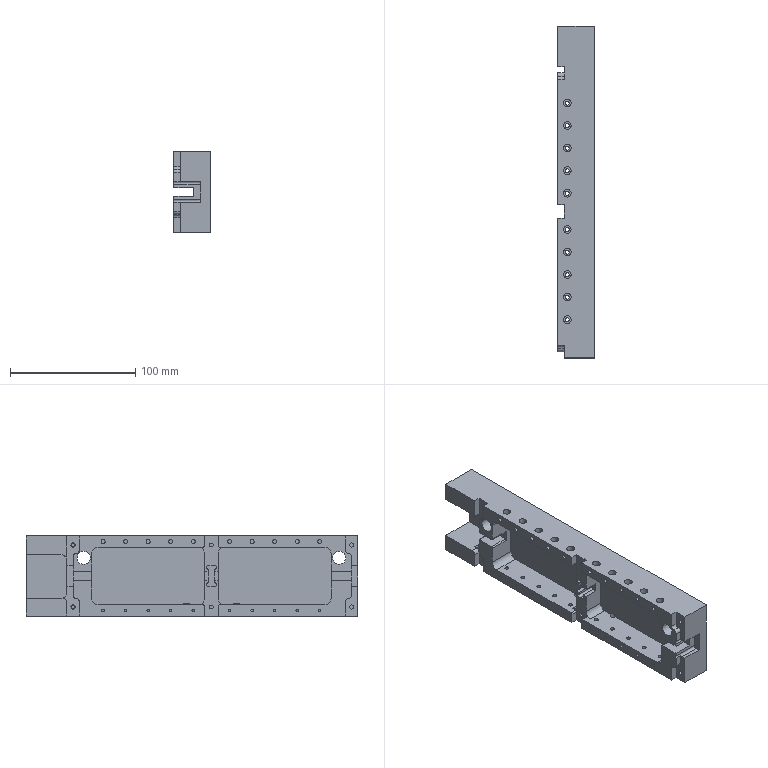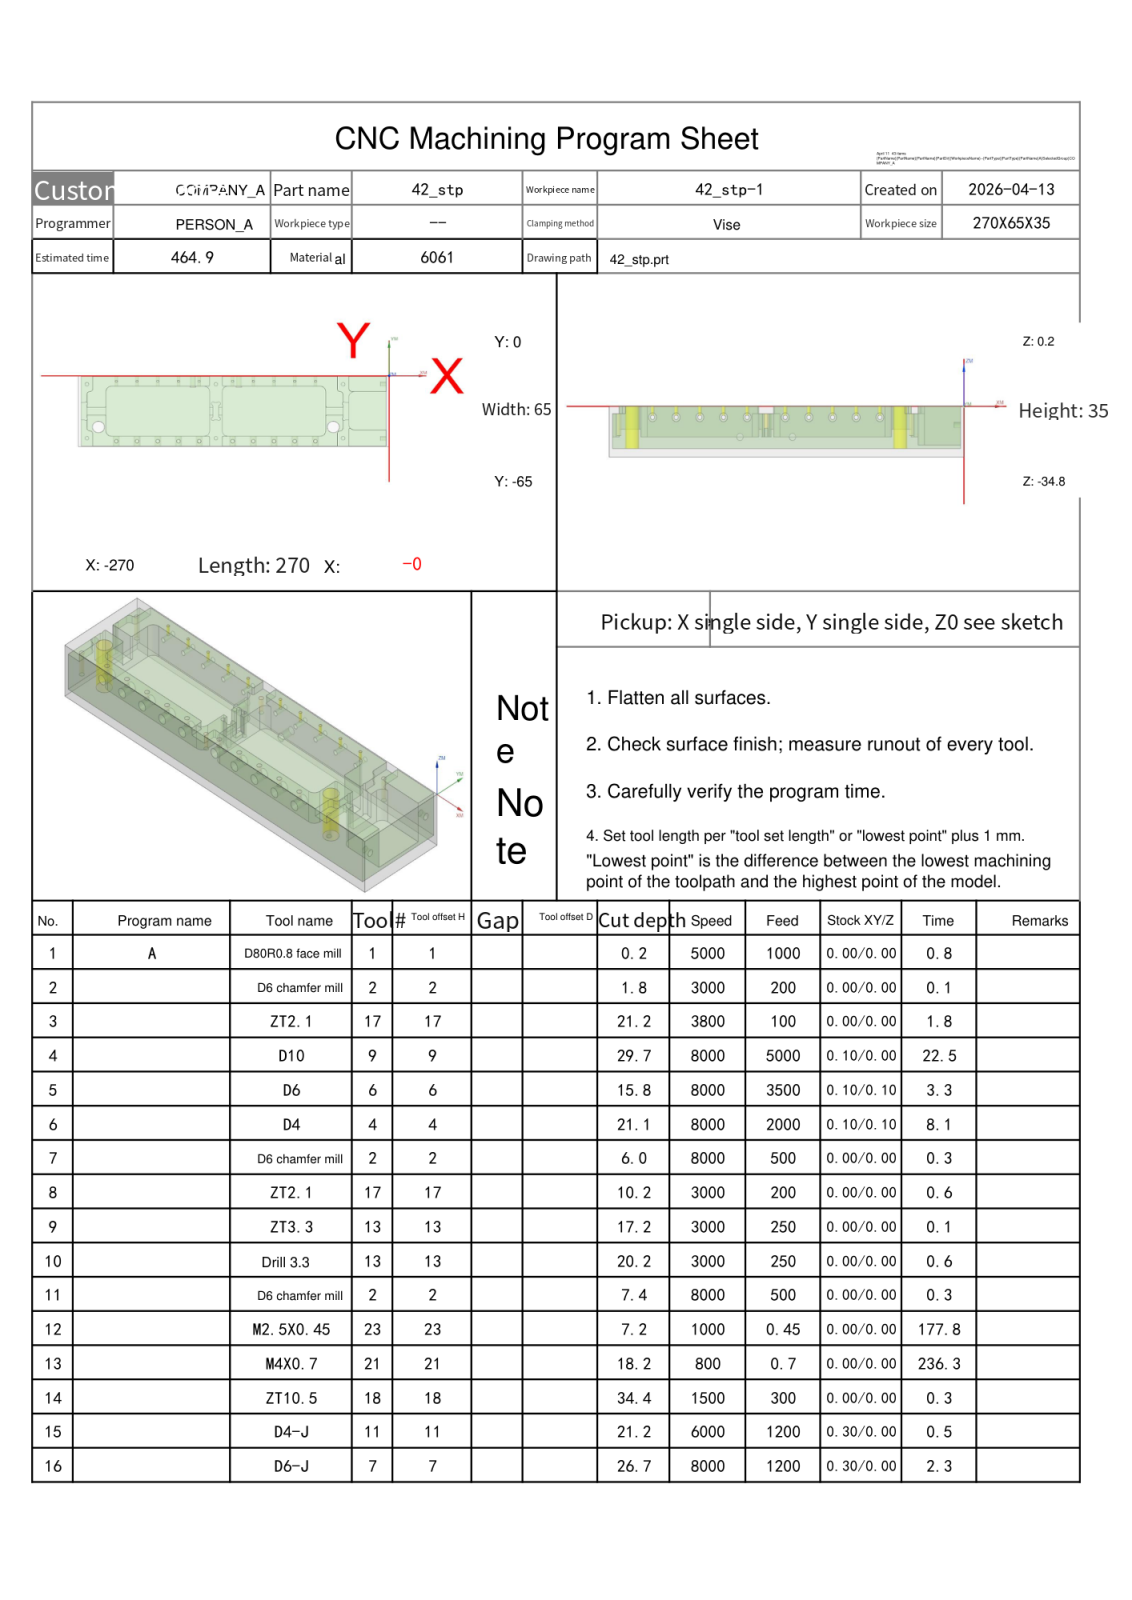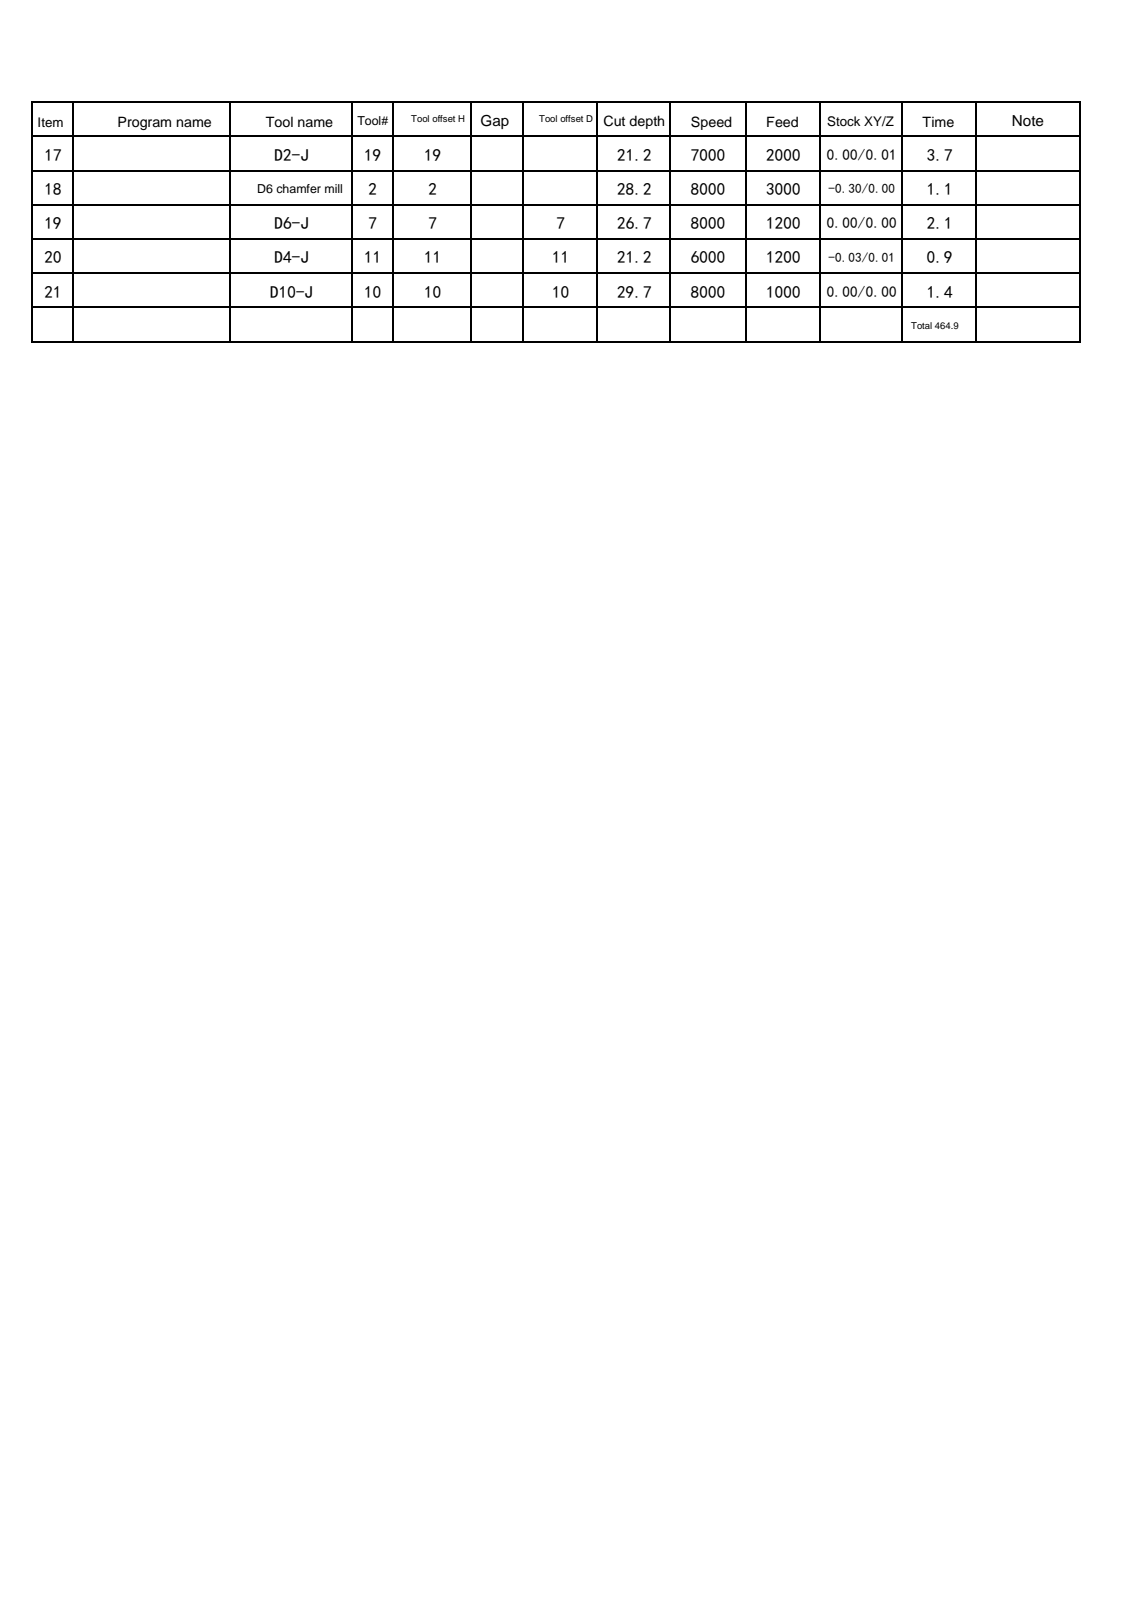NC program | NX | posted by the shop | part box 29 x 265 x 64 mm
Lines 4066 to 6964 of 41846, first 1762 of 2899 lines:
N5 T06 M06
(D6  D=6. R=0. H=06 ce=0.10 di=0.10)
G00 G90 G54 X-162. Y-32.5 M03 S8000
G43 H06 Z10.2
M08
Z1.01
G01 Z-.49 F3000.
X-158.94
Y-14.5
G03 X-160.204 Y-12.6 I-2.06 J0.0
G01 X-157.05
G03 X-153.079 Y-9.522 I0.0 J4.1
G02 X-152.578 Y-9.134 I.501 J-.129
G01 X-152.48 Y-9.143
X-152.325 Y-9.173
X-152.212 Y-9.184
G03 X-151.723 Y-8.931 I0.0 J.6
G02 X-150.5 Y-8.3 I1.223 J-.869
X-149. Y-9.8 I0.0 J-1.5
G01 Y-12.8
G02 X-150.5 Y-14.3 I-1.5 J0.0
X-152. Y-12.8 I0.0 J1.5
G01 Y-10.87
G03 X-152.507 Y-10.278 I-.6 J0.0
G01 X-152.591 Y-10.264
G02 X-153.098 Y-9.672 I.093 J.593
G01 X-153.079 Y-9.522
G03 X-152.95 Y-8.5 I-3.971 J1.022
G01 Y2.44
X-148.05
Y-8.5
G03 X-143.95 Y-12.6 I4.1 J0.0
G01 X-140.796
G03 X-142.06 Y-14.5 I.796 J-1.9
G01 Y-50.5
G03 X-140.796 Y-52.4 I2.06 J0.0
G01 X-143.95
G03 X-147.921 Y-55.478 I0.0 J-4.1
G02 X-148.422 Y-55.866 I-.501 J.129
G01 X-148.52 Y-55.857
X-148.675 Y-55.827
X-148.788 Y-55.816
G03 X-149.277 Y-56.069 I0.0 J-.6
G02 X-150.5 Y-56.7 I-1.223 J.869
X-152. Y-55.2 I0.0 J1.5
G01 Y-52.2
G02 X-150.5 Y-50.7 I1.5 J0.0
X-149. Y-52.2 I0.0 J-1.5
G01 Y-54.13
G03 X-148.493 Y-54.722 I.6 J0.0
G01 X-148.409 Y-54.736
G02 X-147.902 Y-55.328 I-.093 J-.593
G01 X-147.921 Y-55.478
G03 X-148.05 Y-56.5 I3.971 J-1.022
G01 Y-67.44
X-152.95
Y-56.5
G03 X-157.05 Y-52.4 I-4.1 J0.0
G01 X-160.204
G03 X-158.94 Y-50.5 I-.796 J1.9
G01 Y-34.321
G02 X-158.673 Y-33.822 I.6 J0.0
G01 X-154.707 Y-31.178
G03 X-154.44 Y-30.679 I-.333 J.499
G01 Y-17.12
G02 X-154.051 Y-16.56 I.6 J-.002
G03 X-150.926 Y-14.538 I-2.999 J8.06
G02 X-150.5 Y-14.36 I.426 J-.422
X-150.074 Y-14.538 I0.0 J-.6
G03 X-146.949 Y-16.56 I6.124 J6.038
G02 X-146.56 Y-17.12 I-.211 J-.562
G01 Y-47.88
G02 X-146.949 Y-48.44 I-.6 J.002
G03 X-150.074 Y-50.462 I2.999 J-8.06
G02 X-150.5 Y-50.64 I-.426 J.422
X-150.926 Y-50.462 I0.0 J.6
G03 X-154.051 Y-48.44 I-6.124 J-6.038
G02 X-154.44 Y-47.88 I.211 J.562
G01 Y-34.098
G02 X-154.264 Y-33.674 I.6 J0.0
G01 X-151.916 Y-31.326
G03 X-151.74 Y-30.901 I-.424 J.424
G01 Y-18.827
G02 X-151.44 Y-18.309 I.6 J-.002
G03 X-150.829 Y-17.933 I-5.61 J9.809
G02 X-150.5 Y-17.835 I.329 J-.502
X-150.171 Y-17.933 I0.0 J-.6
G03 X-149.56 Y-18.309 I6.221 J9.433
G02 X-149.26 Y-18.827 I-.3 J-.52
G01 Y-46.173
G02 X-149.56 Y-46.691 I-.6 J.002
G03 X-150.171 Y-47.067 I5.61 J-9.809
G02 X-150.5 Y-47.165 I-.329 J.502
X-150.829 Y-47.067 I0.0 J.6
G03 X-151.44 Y-46.691 I-6.221 J-9.433
G02 X-151.74 Y-46.173 I.3 J.52
G01 Y-32.5
Y-32.
X-162.
Z1.01
G00 Y-32.5
Z.52
G01 Z-.98
X-158.94
Y-14.5
G03 X-160.204 Y-12.6 I-2.06 J0.0
G01 X-157.05
G03 X-153.079 Y-9.522 I0.0 J4.1
G02 X-152.578 Y-9.134 I.501 J-.129
G01 X-152.48 Y-9.143
X-152.325 Y-9.173
X-152.212 Y-9.184
G03 X-151.723 Y-8.931 I0.0 J.6
G02 X-150.5 Y-8.3 I1.223 J-.869
X-149. Y-9.8 I0.0 J-1.5
G01 Y-12.8
G02 X-150.5 Y-14.3 I-1.5 J0.0
X-152. Y-12.8 I0.0 J1.5
G01 Y-10.87
G03 X-152.507 Y-10.278 I-.6 J0.0
G01 X-152.591 Y-10.264
G02 X-153.098 Y-9.672 I.093 J.593
G01 X-153.079 Y-9.522
G03 X-152.95 Y-8.5 I-3.971 J1.022
G01 Y2.44
X-148.05
Y-8.5
G03 X-143.95 Y-12.6 I4.1 J0.0
G01 X-140.796
G03 X-142.06 Y-14.5 I.796 J-1.9
G01 Y-50.5
G03 X-140.796 Y-52.4 I2.06 J0.0
G01 X-143.95
G03 X-147.921 Y-55.478 I0.0 J-4.1
G02 X-148.422 Y-55.866 I-.501 J.129
G01 X-148.52 Y-55.857
X-148.675 Y-55.827
X-148.788 Y-55.816
G03 X-149.277 Y-56.069 I0.0 J-.6
G02 X-150.5 Y-56.7 I-1.223 J.869
X-152. Y-55.2 I0.0 J1.5
G01 Y-52.2
G02 X-150.5 Y-50.7 I1.5 J0.0
X-149. Y-52.2 I0.0 J-1.5
G01 Y-54.13
G03 X-148.493 Y-54.722 I.6 J0.0
G01 X-148.409 Y-54.736
G02 X-147.902 Y-55.328 I-.093 J-.593
G01 X-147.921 Y-55.478
G03 X-148.05 Y-56.5 I3.971 J-1.022
G01 Y-67.44
X-152.95
Y-56.5
G03 X-157.05 Y-52.4 I-4.1 J0.0
G01 X-160.204
G03 X-158.94 Y-50.5 I-.796 J1.9
G01 Y-34.321
G02 X-158.673 Y-33.822 I.6 J0.0
G01 X-154.707 Y-31.178
G03 X-154.44 Y-30.679 I-.333 J.499
G01 Y-17.12
G02 X-154.051 Y-16.56 I.6 J-.002
G03 X-150.926 Y-14.538 I-2.999 J8.06
G02 X-150.5 Y-14.36 I.426 J-.422
X-150.074 Y-14.538 I0.0 J-.6
G03 X-146.949 Y-16.56 I6.124 J6.038
G02 X-146.56 Y-17.12 I-.211 J-.562
G01 Y-47.88
G02 X-146.949 Y-48.44 I-.6 J.002
G03 X-150.074 Y-50.462 I2.999 J-8.06
G02 X-150.5 Y-50.64 I-.426 J.422
X-150.926 Y-50.462 I0.0 J.6
G03 X-154.051 Y-48.44 I-6.124 J-6.038
G02 X-154.44 Y-47.88 I.211 J.562
G01 Y-34.098
G02 X-154.264 Y-33.674 I.6 J0.0
G01 X-151.916 Y-31.326
G03 X-151.74 Y-30.901 I-.424 J.424
G01 Y-18.827
G02 X-151.44 Y-18.309 I.6 J-.002
G03 X-150.829 Y-17.933 I-5.61 J9.809
G02 X-150.5 Y-17.835 I.329 J-.502
X-150.171 Y-17.933 I0.0 J-.6
G03 X-149.56 Y-18.309 I6.221 J9.433
G02 X-149.26 Y-18.827 I-.3 J-.52
G01 Y-46.173
G02 X-149.56 Y-46.691 I-.6 J.002
G03 X-150.171 Y-47.067 I5.61 J-9.809
G02 X-150.5 Y-47.165 I-.329 J.502
X-150.829 Y-47.067 I0.0 J.6
G03 X-151.44 Y-46.691 I-6.221 J-9.433
G02 X-151.74 Y-46.173 I.3 J.52
G01 Y-32.5
Y-32.
X-162.
Z.52
G00 Y-32.5
Z.03
G01 Z-1.47
X-158.94
Y-14.5
G03 X-160.204 Y-12.6 I-2.06 J0.0
G01 X-157.05
G03 X-153.079 Y-9.522 I0.0 J4.1
G02 X-152.578 Y-9.134 I.501 J-.129
G01 X-152.48 Y-9.143
X-152.325 Y-9.173
X-152.212 Y-9.184
G03 X-151.723 Y-8.931 I0.0 J.6
G02 X-150.5 Y-8.3 I1.223 J-.869
X-149. Y-9.8 I0.0 J-1.5
G01 Y-12.8
G02 X-150.5 Y-14.3 I-1.5 J0.0
X-152. Y-12.8 I0.0 J1.5
G01 Y-10.87
G03 X-152.507 Y-10.278 I-.6 J0.0
G01 X-152.591 Y-10.264
G02 X-153.098 Y-9.672 I.093 J.593
G01 X-153.079 Y-9.522
G03 X-152.95 Y-8.5 I-3.971 J1.022
G01 Y2.44
X-148.05
Y-8.5
G03 X-143.95 Y-12.6 I4.1 J0.0
G01 X-140.796
G03 X-142.06 Y-14.5 I.796 J-1.9
G01 Y-50.5
G03 X-140.796 Y-52.4 I2.06 J0.0
G01 X-143.95
G03 X-147.921 Y-55.478 I0.0 J-4.1
G02 X-148.422 Y-55.866 I-.501 J.129
G01 X-148.52 Y-55.857
X-148.675 Y-55.827
X-148.788 Y-55.816
G03 X-149.277 Y-56.069 I0.0 J-.6
G02 X-150.5 Y-56.7 I-1.223 J.869
X-152. Y-55.2 I0.0 J1.5
G01 Y-52.2
G02 X-150.5 Y-50.7 I1.5 J0.0
X-149. Y-52.2 I0.0 J-1.5
G01 Y-54.13
G03 X-148.493 Y-54.722 I.6 J0.0
G01 X-148.409 Y-54.736
G02 X-147.902 Y-55.328 I-.093 J-.593
G01 X-147.921 Y-55.478
G03 X-148.05 Y-56.5 I3.971 J-1.022
G01 Y-67.44
X-152.95
Y-56.5
G03 X-157.05 Y-52.4 I-4.1 J0.0
G01 X-160.204
G03 X-158.94 Y-50.5 I-.796 J1.9
G01 Y-34.321
G02 X-158.673 Y-33.822 I.6 J0.0
G01 X-154.707 Y-31.178
G03 X-154.44 Y-30.679 I-.333 J.499
G01 Y-17.12
G02 X-154.051 Y-16.56 I.6 J-.002
G03 X-150.926 Y-14.538 I-2.999 J8.06
G02 X-150.5 Y-14.36 I.426 J-.422
X-150.074 Y-14.538 I0.0 J-.6
G03 X-146.949 Y-16.56 I6.124 J6.038
G02 X-146.56 Y-17.12 I-.211 J-.562
G01 Y-47.88
G02 X-146.949 Y-48.44 I-.6 J.002
G03 X-150.074 Y-50.462 I2.999 J-8.06
G02 X-150.5 Y-50.64 I-.426 J.422
X-150.926 Y-50.462 I0.0 J.6
G03 X-154.051 Y-48.44 I-6.124 J-6.038
G02 X-154.44 Y-47.88 I.211 J.562
G01 Y-34.098
G02 X-154.264 Y-33.674 I.6 J0.0
G01 X-151.916 Y-31.326
G03 X-151.74 Y-30.901 I-.424 J.424
G01 Y-18.827
G02 X-151.44 Y-18.309 I.6 J-.002
G03 X-150.829 Y-17.933 I-5.61 J9.809
G02 X-150.5 Y-17.835 I.329 J-.502
X-150.171 Y-17.933 I0.0 J-.6
G03 X-149.56 Y-18.309 I6.221 J9.433
G02 X-149.26 Y-18.827 I-.3 J-.52
G01 Y-46.173
G02 X-149.56 Y-46.691 I-.6 J.002
G03 X-150.171 Y-47.067 I5.61 J-9.809
G02 X-150.5 Y-47.165 I-.329 J.502
X-150.829 Y-47.067 I0.0 J.6
G03 X-151.44 Y-46.691 I-6.221 J-9.433
G02 X-151.74 Y-46.173 I.3 J.52
G01 Y-32.5
Y-32.
X-162.
Z.03
G00 Y-32.5
Z-.46
G01 Z-1.96
X-158.94
Y-14.5
G03 X-160.204 Y-12.6 I-2.06 J0.0
G01 X-157.05
G03 X-153.079 Y-9.522 I0.0 J4.1
G02 X-152.578 Y-9.134 I.501 J-.129
G01 X-152.48 Y-9.143
X-152.325 Y-9.173
X-152.212 Y-9.184
G03 X-151.723 Y-8.931 I0.0 J.6
G02 X-150.5 Y-8.3 I1.223 J-.869
X-149. Y-9.8 I0.0 J-1.5
G01 Y-12.8
G02 X-150.5 Y-14.3 I-1.5 J0.0
X-152. Y-12.8 I0.0 J1.5
G01 Y-10.87
G03 X-152.507 Y-10.278 I-.6 J0.0
G01 X-152.591 Y-10.264
G02 X-153.098 Y-9.672 I.093 J.593
G01 X-153.079 Y-9.522
G03 X-152.95 Y-8.5 I-3.971 J1.022
G01 Y2.44
X-148.05
Y-8.5
G03 X-143.95 Y-12.6 I4.1 J0.0
G01 X-140.796
G03 X-142.06 Y-14.5 I.796 J-1.9
G01 Y-50.5
G03 X-140.796 Y-52.4 I2.06 J0.0
G01 X-143.95
G03 X-147.921 Y-55.478 I0.0 J-4.1
G02 X-148.422 Y-55.866 I-.501 J.129
G01 X-148.52 Y-55.857
X-148.675 Y-55.827
X-148.788 Y-55.816
G03 X-149.277 Y-56.069 I0.0 J-.6
G02 X-150.5 Y-56.7 I-1.223 J.869
X-152. Y-55.2 I0.0 J1.5
G01 Y-52.2
G02 X-150.5 Y-50.7 I1.5 J0.0
X-149. Y-52.2 I0.0 J-1.5
G01 Y-54.13
G03 X-148.493 Y-54.722 I.6 J0.0
G01 X-148.409 Y-54.736
G02 X-147.902 Y-55.328 I-.093 J-.593
G01 X-147.921 Y-55.478
G03 X-148.05 Y-56.5 I3.971 J-1.022
G01 Y-67.44
X-152.95
Y-56.5
G03 X-157.05 Y-52.4 I-4.1 J0.0
G01 X-160.204
G03 X-158.94 Y-50.5 I-.796 J1.9
G01 Y-34.321
G02 X-158.673 Y-33.822 I.6 J0.0
G01 X-154.707 Y-31.178
G03 X-154.44 Y-30.679 I-.333 J.499
G01 Y-17.12
G02 X-154.051 Y-16.56 I.6 J-.002
G03 X-150.926 Y-14.538 I-2.999 J8.06
G02 X-150.5 Y-14.36 I.426 J-.422
X-150.074 Y-14.538 I0.0 J-.6
G03 X-146.949 Y-16.56 I6.124 J6.038
G02 X-146.56 Y-17.12 I-.211 J-.562
G01 Y-47.88
G02 X-146.949 Y-48.44 I-.6 J.002
G03 X-150.074 Y-50.462 I2.999 J-8.06
G02 X-150.5 Y-50.64 I-.426 J.422
X-150.926 Y-50.462 I0.0 J.6
G03 X-154.051 Y-48.44 I-6.124 J-6.038
G02 X-154.44 Y-47.88 I.211 J.562
G01 Y-34.098
G02 X-154.264 Y-33.674 I.6 J0.0
G01 X-151.916 Y-31.326
G03 X-151.74 Y-30.901 I-.424 J.424
G01 Y-18.827
G02 X-151.44 Y-18.309 I.6 J-.002
G03 X-150.829 Y-17.933 I-5.61 J9.809
G02 X-150.5 Y-17.835 I.329 J-.502
X-150.171 Y-17.933 I0.0 J-.6
G03 X-149.56 Y-18.309 I6.221 J9.433
G02 X-149.26 Y-18.827 I-.3 J-.52
G01 Y-46.173
G02 X-149.56 Y-46.691 I-.6 J.002
G03 X-150.171 Y-47.067 I5.61 J-9.809
G02 X-150.5 Y-47.165 I-.329 J.502
X-150.829 Y-47.067 I0.0 J.6
G03 X-151.44 Y-46.691 I-6.221 J-9.433
G02 X-151.74 Y-46.173 I.3 J.52
G01 Y-32.5
Y-32.
X-162.
Z-.46
G00 Y-32.5
Z-.95
G01 Z-2.45
X-158.94
Y-14.5
G03 X-160.204 Y-12.6 I-2.06 J0.0
G01 X-157.05
G03 X-153.079 Y-9.522 I0.0 J4.1
G02 X-152.578 Y-9.134 I.501 J-.129
G01 X-152.48 Y-9.143
X-152.325 Y-9.173
X-152.212 Y-9.184
G03 X-151.723 Y-8.931 I0.0 J.6
G02 X-150.5 Y-8.3 I1.223 J-.869
X-149. Y-9.8 I0.0 J-1.5
G01 Y-12.8
G02 X-150.5 Y-14.3 I-1.5 J0.0
X-152. Y-12.8 I0.0 J1.5
G01 Y-10.87
G03 X-152.507 Y-10.278 I-.6 J0.0
G01 X-152.591 Y-10.264
G02 X-153.098 Y-9.672 I.093 J.593
G01 X-153.079 Y-9.522
G03 X-152.95 Y-8.5 I-3.971 J1.022
G01 Y2.44
X-148.05
Y-8.5
G03 X-143.95 Y-12.6 I4.1 J0.0
G01 X-140.796
G03 X-142.06 Y-14.5 I.796 J-1.9
G01 Y-50.5
G03 X-140.796 Y-52.4 I2.06 J0.0
G01 X-143.95
G03 X-147.921 Y-55.478 I0.0 J-4.1
G02 X-148.422 Y-55.866 I-.501 J.129
G01 X-148.52 Y-55.857
X-148.675 Y-55.827
X-148.788 Y-55.816
G03 X-149.277 Y-56.069 I0.0 J-.6
G02 X-150.5 Y-56.7 I-1.223 J.869
X-152. Y-55.2 I0.0 J1.5
G01 Y-52.2
G02 X-150.5 Y-50.7 I1.5 J0.0
X-149. Y-52.2 I0.0 J-1.5
G01 Y-54.13
G03 X-148.493 Y-54.722 I.6 J0.0
G01 X-148.409 Y-54.736
G02 X-147.902 Y-55.328 I-.093 J-.593
G01 X-147.921 Y-55.478
G03 X-148.05 Y-56.5 I3.971 J-1.022
G01 Y-67.44
X-152.95
Y-56.5
G03 X-157.05 Y-52.4 I-4.1 J0.0
G01 X-160.204
G03 X-158.94 Y-50.5 I-.796 J1.9
G01 Y-34.321
G02 X-158.673 Y-33.822 I.6 J0.0
G01 X-154.707 Y-31.178
G03 X-154.44 Y-30.679 I-.333 J.499
G01 Y-17.12
G02 X-154.051 Y-16.56 I.6 J-.002
G03 X-150.926 Y-14.538 I-2.999 J8.06
G02 X-150.5 Y-14.36 I.426 J-.422
X-150.074 Y-14.538 I0.0 J-.6
G03 X-146.949 Y-16.56 I6.124 J6.038
G02 X-146.56 Y-17.12 I-.211 J-.562
G01 Y-47.88
G02 X-146.949 Y-48.44 I-.6 J.002
G03 X-150.074 Y-50.462 I2.999 J-8.06
G02 X-150.5 Y-50.64 I-.426 J.422
X-150.926 Y-50.462 I0.0 J.6
G03 X-154.051 Y-48.44 I-6.124 J-6.038
G02 X-154.44 Y-47.88 I.211 J.562
G01 Y-34.098
G02 X-154.264 Y-33.674 I.6 J0.0
G01 X-151.916 Y-31.326
G03 X-151.74 Y-30.901 I-.424 J.424
G01 Y-18.827
G02 X-151.44 Y-18.309 I.6 J-.002
G03 X-150.829 Y-17.933 I-5.61 J9.809
G02 X-150.5 Y-17.835 I.329 J-.502
X-150.171 Y-17.933 I0.0 J-.6
G03 X-149.56 Y-18.309 I6.221 J9.433
G02 X-149.26 Y-18.827 I-.3 J-.52
G01 Y-46.173
G02 X-149.56 Y-46.691 I-.6 J.002
G03 X-150.171 Y-47.067 I5.61 J-9.809
G02 X-150.5 Y-47.165 I-.329 J.502
X-150.829 Y-47.067 I0.0 J.6
G03 X-151.44 Y-46.691 I-6.221 J-9.433
G02 X-151.74 Y-46.173 I.3 J.52
G01 Y-32.5
Y-32.
X-162.
Z-.95
G00 Y-32.5
Z-1.44
G01 Z-2.94
X-158.94
Y-14.5
G03 X-160.204 Y-12.6 I-2.06 J0.0
G01 X-157.05
G03 X-153.079 Y-9.522 I0.0 J4.1
G02 X-152.578 Y-9.134 I.501 J-.129
G01 X-152.48 Y-9.143
X-152.325 Y-9.173
X-152.212 Y-9.184
G03 X-151.723 Y-8.931 I0.0 J.6
G02 X-150.5 Y-8.3 I1.223 J-.869
X-149. Y-9.8 I0.0 J-1.5
G01 Y-12.8
G02 X-150.5 Y-14.3 I-1.5 J0.0
X-152. Y-12.8 I0.0 J1.5
G01 Y-10.87
G03 X-152.507 Y-10.278 I-.6 J0.0
G01 X-152.591 Y-10.264
G02 X-153.098 Y-9.672 I.093 J.593
G01 X-153.079 Y-9.522
G03 X-152.95 Y-8.5 I-3.971 J1.022
G01 Y2.44
X-148.05
Y-8.5
G03 X-143.95 Y-12.6 I4.1 J0.0
G01 X-140.796
G03 X-142.06 Y-14.5 I.796 J-1.9
G01 Y-50.5
G03 X-140.796 Y-52.4 I2.06 J0.0
G01 X-143.95
G03 X-147.921 Y-55.478 I0.0 J-4.1
G02 X-148.422 Y-55.866 I-.501 J.129
G01 X-148.52 Y-55.857
X-148.675 Y-55.827
X-148.788 Y-55.816
G03 X-149.277 Y-56.069 I0.0 J-.6
G02 X-150.5 Y-56.7 I-1.223 J.869
X-152. Y-55.2 I0.0 J1.5
G01 Y-52.2
G02 X-150.5 Y-50.7 I1.5 J0.0
X-149. Y-52.2 I0.0 J-1.5
G01 Y-54.13
G03 X-148.493 Y-54.722 I.6 J0.0
G01 X-148.409 Y-54.736
G02 X-147.902 Y-55.328 I-.093 J-.593
G01 X-147.921 Y-55.478
G03 X-148.05 Y-56.5 I3.971 J-1.022
G01 Y-67.44
X-152.95
Y-56.5
G03 X-157.05 Y-52.4 I-4.1 J0.0
G01 X-160.204
G03 X-158.94 Y-50.5 I-.796 J1.9
G01 Y-34.321
G02 X-158.673 Y-33.822 I.6 J0.0
G01 X-154.707 Y-31.178
G03 X-154.44 Y-30.679 I-.333 J.499
G01 Y-17.12
G02 X-154.051 Y-16.56 I.6 J-.002
G03 X-150.926 Y-14.538 I-2.999 J8.06
G02 X-150.5 Y-14.36 I.426 J-.422
X-150.074 Y-14.538 I0.0 J-.6
G03 X-146.949 Y-16.56 I6.124 J6.038
G02 X-146.56 Y-17.12 I-.211 J-.562
G01 Y-47.88
G02 X-146.949 Y-48.44 I-.6 J.002
G03 X-150.074 Y-50.462 I2.999 J-8.06
G02 X-150.5 Y-50.64 I-.426 J.422
X-150.926 Y-50.462 I0.0 J.6
G03 X-154.051 Y-48.44 I-6.124 J-6.038
G02 X-154.44 Y-47.88 I.211 J.562
G01 Y-34.098
G02 X-154.264 Y-33.674 I.6 J0.0
G01 X-151.916 Y-31.326
G03 X-151.74 Y-30.901 I-.424 J.424
G01 Y-18.827
G02 X-151.44 Y-18.309 I.6 J-.002
G03 X-150.829 Y-17.933 I-5.61 J9.809
G02 X-150.5 Y-17.835 I.329 J-.502
X-150.171 Y-17.933 I0.0 J-.6
G03 X-149.56 Y-18.309 I6.221 J9.433
G02 X-149.26 Y-18.827 I-.3 J-.52
G01 Y-46.173
G02 X-149.56 Y-46.691 I-.6 J.002
G03 X-150.171 Y-47.067 I5.61 J-9.809
G02 X-150.5 Y-47.165 I-.329 J.502
X-150.829 Y-47.067 I0.0 J.6
G03 X-151.44 Y-46.691 I-6.221 J-9.433
G02 X-151.74 Y-46.173 I.3 J.52
G01 Y-32.5
Y-32.
X-162.
Z-1.44
G00 Y-32.5
Z-1.93
G01 Z-3.43
X-158.94
Y-14.5
G03 X-160.204 Y-12.6 I-2.06 J0.0
G01 X-157.05
G03 X-153.079 Y-9.522 I0.0 J4.1
G02 X-152.578 Y-9.134 I.501 J-.129
G01 X-152.48 Y-9.143
X-152.325 Y-9.173
X-152.212 Y-9.184
G03 X-151.723 Y-8.931 I0.0 J.6
G02 X-150.5 Y-8.3 I1.223 J-.869
X-149. Y-9.8 I0.0 J-1.5
G01 Y-12.8
G02 X-150.5 Y-14.3 I-1.5 J0.0
X-152. Y-12.8 I0.0 J1.5
G01 Y-10.87
G03 X-152.507 Y-10.278 I-.6 J0.0
G01 X-152.591 Y-10.264
G02 X-153.098 Y-9.672 I.093 J.593
G01 X-153.079 Y-9.522
G03 X-152.95 Y-8.5 I-3.971 J1.022
G01 Y2.44
X-148.05
Y-8.5
G03 X-143.95 Y-12.6 I4.1 J0.0
G01 X-140.796
G03 X-142.06 Y-14.5 I.796 J-1.9
G01 Y-50.5
G03 X-140.796 Y-52.4 I2.06 J0.0
G01 X-143.95
G03 X-147.921 Y-55.478 I0.0 J-4.1
G02 X-148.422 Y-55.866 I-.501 J.129
G01 X-148.52 Y-55.857
X-148.675 Y-55.827
X-148.788 Y-55.816
G03 X-149.277 Y-56.069 I0.0 J-.6
G02 X-150.5 Y-56.7 I-1.223 J.869
X-152. Y-55.2 I0.0 J1.5
G01 Y-52.2
G02 X-150.5 Y-50.7 I1.5 J0.0
X-149. Y-52.2 I0.0 J-1.5
G01 Y-54.13
G03 X-148.493 Y-54.722 I.6 J0.0
G01 X-148.409 Y-54.736
G02 X-147.902 Y-55.328 I-.093 J-.593
G01 X-147.921 Y-55.478
G03 X-148.05 Y-56.5 I3.971 J-1.022
G01 Y-67.44
X-152.95
Y-56.5
G03 X-157.05 Y-52.4 I-4.1 J0.0
G01 X-160.204
G03 X-158.94 Y-50.5 I-.796 J1.9
G01 Y-34.321
G02 X-158.673 Y-33.822 I.6 J0.0
G01 X-154.707 Y-31.178
G03 X-154.44 Y-30.679 I-.333 J.499
G01 Y-17.12
G02 X-154.051 Y-16.56 I.6 J-.002
G03 X-150.926 Y-14.538 I-2.999 J8.06
G02 X-150.5 Y-14.36 I.426 J-.422
X-150.074 Y-14.538 I0.0 J-.6
G03 X-146.949 Y-16.56 I6.124 J6.038
G02 X-146.56 Y-17.12 I-.211 J-.562
G01 Y-47.88
G02 X-146.949 Y-48.44 I-.6 J.002
G03 X-150.074 Y-50.462 I2.999 J-8.06
G02 X-150.5 Y-50.64 I-.426 J.422
X-150.926 Y-50.462 I0.0 J.6
G03 X-154.051 Y-48.44 I-6.124 J-6.038
G02 X-154.44 Y-47.88 I.211 J.562
G01 Y-34.098
G02 X-154.264 Y-33.674 I.6 J0.0
G01 X-151.916 Y-31.326
G03 X-151.74 Y-30.901 I-.424 J.424
G01 Y-18.827
G02 X-151.44 Y-18.309 I.6 J-.002
G03 X-150.829 Y-17.933 I-5.61 J9.809
G02 X-150.5 Y-17.835 I.329 J-.502
X-150.171 Y-17.933 I0.0 J-.6
G03 X-149.56 Y-18.309 I6.221 J9.433
G02 X-149.26 Y-18.827 I-.3 J-.52
G01 Y-46.173
G02 X-149.56 Y-46.691 I-.6 J.002
G03 X-150.171 Y-47.067 I5.61 J-9.809
G02 X-150.5 Y-47.165 I-.329 J.502
X-150.829 Y-47.067 I0.0 J.6
G03 X-151.44 Y-46.691 I-6.221 J-9.433
G02 X-151.74 Y-46.173 I.3 J.52
G01 Y-32.5
Y-32.
X-162.
Z-1.93
G00 Y-32.5
Z-2.42
G01 Z-3.92
X-158.94
Y-14.5
G03 X-160.204 Y-12.6 I-2.06 J0.0
G01 X-157.05
G03 X-153.079 Y-9.522 I0.0 J4.1
G02 X-152.578 Y-9.134 I.501 J-.129
G01 X-152.48 Y-9.143
X-152.325 Y-9.173
X-152.212 Y-9.184
G03 X-151.723 Y-8.931 I0.0 J.6
G02 X-150.5 Y-8.3 I1.223 J-.869
X-149. Y-9.8 I0.0 J-1.5
G01 Y-12.8
G02 X-150.5 Y-14.3 I-1.5 J0.0
X-152. Y-12.8 I0.0 J1.5
G01 Y-10.87
G03 X-152.507 Y-10.278 I-.6 J0.0
G01 X-152.591 Y-10.264
G02 X-153.098 Y-9.672 I.093 J.593
G01 X-153.079 Y-9.522
G03 X-152.95 Y-8.5 I-3.971 J1.022
G01 Y2.44
X-148.05
Y-8.5
G03 X-143.95 Y-12.6 I4.1 J0.0
G01 X-140.796
G03 X-142.06 Y-14.5 I.796 J-1.9
G01 Y-50.5
G03 X-140.796 Y-52.4 I2.06 J0.0
G01 X-143.95
G03 X-147.921 Y-55.478 I0.0 J-4.1
G02 X-148.422 Y-55.866 I-.501 J.129
G01 X-148.52 Y-55.857
X-148.675 Y-55.827
X-148.788 Y-55.816
G03 X-149.277 Y-56.069 I0.0 J-.6
G02 X-150.5 Y-56.7 I-1.223 J.869
X-152. Y-55.2 I0.0 J1.5
G01 Y-52.2
G02 X-150.5 Y-50.7 I1.5 J0.0
X-149. Y-52.2 I0.0 J-1.5
G01 Y-54.13
G03 X-148.493 Y-54.722 I.6 J0.0
G01 X-148.409 Y-54.736
G02 X-147.902 Y-55.328 I-.093 J-.593
G01 X-147.921 Y-55.478
G03 X-148.05 Y-56.5 I3.971 J-1.022
G01 Y-67.44
X-152.95
Y-56.5
G03 X-157.05 Y-52.4 I-4.1 J0.0
G01 X-160.204
G03 X-158.94 Y-50.5 I-.796 J1.9
G01 Y-34.321
G02 X-158.673 Y-33.822 I.6 J0.0
G01 X-154.707 Y-31.178
G03 X-154.44 Y-30.679 I-.333 J.499
G01 Y-17.12
G02 X-154.051 Y-16.56 I.6 J-.002
G03 X-150.926 Y-14.538 I-2.999 J8.06
G02 X-150.5 Y-14.36 I.426 J-.422
X-150.074 Y-14.538 I0.0 J-.6
G03 X-146.949 Y-16.56 I6.124 J6.038
G02 X-146.56 Y-17.12 I-.211 J-.562
G01 Y-47.88
G02 X-146.949 Y-48.44 I-.6 J.002
G03 X-150.074 Y-50.462 I2.999 J-8.06
G02 X-150.5 Y-50.64 I-.426 J.422
X-150.926 Y-50.462 I0.0 J.6
G03 X-154.051 Y-48.44 I-6.124 J-6.038
G02 X-154.44 Y-47.88 I.211 J.562
G01 Y-34.098
G02 X-154.264 Y-33.674 I.6 J0.0
G01 X-151.916 Y-31.326
G03 X-151.74 Y-30.901 I-.424 J.424
G01 Y-18.827
G02 X-151.44 Y-18.309 I.6 J-.002
G03 X-150.829 Y-17.933 I-5.61 J9.809
G02 X-150.5 Y-17.835 I.329 J-.502
X-150.171 Y-17.933 I0.0 J-.6
G03 X-149.56 Y-18.309 I6.221 J9.433
G02 X-149.26 Y-18.827 I-.3 J-.52
G01 Y-46.173
G02 X-149.56 Y-46.691 I-.6 J.002
G03 X-150.171 Y-47.067 I5.61 J-9.809
G02 X-150.5 Y-47.165 I-.329 J.502
X-150.829 Y-47.067 I0.0 J.6
G03 X-151.44 Y-46.691 I-6.221 J-9.433
G02 X-151.74 Y-46.173 I.3 J.52
G01 Y-32.5
Y-32.
X-162.
Z-2.42
G00 Y-32.5
Z-2.91
G01 Z-4.41
X-158.94
Y-14.5
G03 X-160.204 Y-12.6 I-2.06 J0.0
G01 X-157.05
G03 X-153.079 Y-9.522 I0.0 J4.1
G02 X-152.578 Y-9.134 I.501 J-.129
G01 X-152.48 Y-9.143
X-152.325 Y-9.173
X-152.212 Y-9.184
G03 X-151.723 Y-8.931 I0.0 J.6
G02 X-150.5 Y-8.3 I1.223 J-.869
X-149. Y-9.8 I0.0 J-1.5
G01 Y-12.8
G02 X-150.5 Y-14.3 I-1.5 J0.0
X-152. Y-12.8 I0.0 J1.5
G01 Y-10.87
G03 X-152.507 Y-10.278 I-.6 J0.0
G01 X-152.591 Y-10.264
G02 X-153.098 Y-9.672 I.093 J.593
G01 X-153.079 Y-9.522
G03 X-152.95 Y-8.5 I-3.971 J1.022
G01 Y2.44
X-148.05
Y-8.5
G03 X-143.95 Y-12.6 I4.1 J0.0
G01 X-140.796
G03 X-142.06 Y-14.5 I.796 J-1.9
G01 Y-50.5
G03 X-140.796 Y-52.4 I2.06 J0.0
G01 X-143.95
G03 X-147.921 Y-55.478 I0.0 J-4.1
G02 X-148.422 Y-55.866 I-.501 J.129
G01 X-148.52 Y-55.857
X-148.675 Y-55.827
X-148.788 Y-55.816
G03 X-149.277 Y-56.069 I0.0 J-.6
G02 X-150.5 Y-56.7 I-1.223 J.869
X-152. Y-55.2 I0.0 J1.5
G01 Y-52.2
G02 X-150.5 Y-50.7 I1.5 J0.0
X-149. Y-52.2 I0.0 J-1.5
G01 Y-54.13
G03 X-148.493 Y-54.722 I.6 J0.0
G01 X-148.409 Y-54.736
G02 X-147.902 Y-55.328 I-.093 J-.593
G01 X-147.921 Y-55.478
G03 X-148.05 Y-56.5 I3.971 J-1.022
G01 Y-67.44
X-152.95
Y-56.5
G03 X-157.05 Y-52.4 I-4.1 J0.0
G01 X-160.204
G03 X-158.94 Y-50.5 I-.796 J1.9
G01 Y-34.321
G02 X-158.673 Y-33.822 I.6 J0.0
G01 X-154.707 Y-31.178
G03 X-154.44 Y-30.679 I-.333 J.499
G01 Y-17.12
G02 X-154.051 Y-16.56 I.6 J-.002
G03 X-150.926 Y-14.538 I-2.999 J8.06
G02 X-150.5 Y-14.36 I.426 J-.422
X-150.074 Y-14.538 I0.0 J-.6
G03 X-146.949 Y-16.56 I6.124 J6.038
G02 X-146.56 Y-17.12 I-.211 J-.562
G01 Y-47.88
G02 X-146.949 Y-48.44 I-.6 J.002
G03 X-150.074 Y-50.462 I2.999 J-8.06
G02 X-150.5 Y-50.64 I-.426 J.422
X-150.926 Y-50.462 I0.0 J.6
G03 X-154.051 Y-48.44 I-6.124 J-6.038
G02 X-154.44 Y-47.88 I.211 J.562
G01 Y-34.098
G02 X-154.264 Y-33.674 I.6 J0.0
G01 X-151.916 Y-31.326
G03 X-151.74 Y-30.901 I-.424 J.424
G01 Y-18.827
G02 X-151.44 Y-18.309 I.6 J-.002
G03 X-150.829 Y-17.933 I-5.61 J9.809
G02 X-150.5 Y-17.835 I.329 J-.502
X-150.171 Y-17.933 I0.0 J-.6
G03 X-149.56 Y-18.309 I6.221 J9.433
G02 X-149.26 Y-18.827 I-.3 J-.52
G01 Y-46.173
G02 X-149.56 Y-46.691 I-.6 J.002
G03 X-150.171 Y-47.067 I5.61 J-9.809
G02 X-150.5 Y-47.165 I-.329 J.502
X-150.829 Y-47.067 I0.0 J.6
G03 X-151.44 Y-46.691 I-6.221 J-9.433
G02 X-151.74 Y-46.173 I.3 J.52
G01 Y-32.5
Y-32.
X-162.
Z-2.91
G00 Y-32.5
Z-3.4
G01 Z-4.9
X-158.94
Y-14.5
G03 X-160.204 Y-12.6 I-2.06 J0.0
G01 X-157.05
G03 X-153.079 Y-9.522 I0.0 J4.1
G02 X-152.578 Y-9.134 I.501 J-.129
G01 X-152.48 Y-9.143
X-152.325 Y-9.173
X-152.212 Y-9.184
G03 X-151.723 Y-8.931 I0.0 J.6
G02 X-150.5 Y-8.3 I1.223 J-.869
X-149. Y-9.8 I0.0 J-1.5
G01 Y-12.8
G02 X-150.5 Y-14.3 I-1.5 J0.0
X-152. Y-12.8 I0.0 J1.5
G01 Y-10.87
G03 X-152.507 Y-10.278 I-.6 J0.0
G01 X-152.591 Y-10.264
G02 X-153.098 Y-9.672 I.093 J.593
G01 X-153.079 Y-9.522
G03 X-152.95 Y-8.5 I-3.971 J1.022
G01 Y2.44
X-148.05
Y-8.5
G03 X-143.95 Y-12.6 I4.1 J0.0
G01 X-140.796
G03 X-142.06 Y-14.5 I.796 J-1.9
G01 Y-50.5
G03 X-140.796 Y-52.4 I2.06 J0.0
G01 X-143.95
G03 X-147.921 Y-55.478 I0.0 J-4.1
G02 X-148.422 Y-55.866 I-.501 J.129
G01 X-148.52 Y-55.857
X-148.675 Y-55.827
X-148.788 Y-55.816
G03 X-149.277 Y-56.069 I0.0 J-.6
G02 X-150.5 Y-56.7 I-1.223 J.869
X-152. Y-55.2 I0.0 J1.5
G01 Y-52.2
G02 X-150.5 Y-50.7 I1.5 J0.0
X-149. Y-52.2 I0.0 J-1.5
G01 Y-54.13
G03 X-148.493 Y-54.722 I.6 J0.0
G01 X-148.409 Y-54.736
G02 X-147.902 Y-55.328 I-.093 J-.593
G01 X-147.921 Y-55.478
G03 X-148.05 Y-56.5 I3.971 J-1.022
G01 Y-67.44
X-152.95
Y-56.5
G03 X-157.05 Y-52.4 I-4.1 J0.0
G01 X-160.204
G03 X-158.94 Y-50.5 I-.796 J1.9
G01 Y-34.321
G02 X-158.673 Y-33.822 I.6 J0.0
G01 X-154.707 Y-31.178
G03 X-154.44 Y-30.679 I-.333 J.499
G01 Y-17.12
G02 X-154.051 Y-16.56 I.6 J-.002
G03 X-150.926 Y-14.538 I-2.999 J8.06
G02 X-150.5 Y-14.36 I.426 J-.422
X-150.074 Y-14.538 I0.0 J-.6
G03 X-146.949 Y-16.56 I6.124 J6.038
G02 X-146.56 Y-17.12 I-.211 J-.562
G01 Y-47.88
G02 X-146.949 Y-48.44 I-.6 J.002
G03 X-150.074 Y-50.462 I2.999 J-8.06
G02 X-150.5 Y-50.64 I-.426 J.422
X-150.926 Y-50.462 I0.0 J.6
G03 X-154.051 Y-48.44 I-6.124 J-6.038
G02 X-154.44 Y-47.88 I.211 J.562
G01 Y-34.098
G02 X-154.264 Y-33.674 I.6 J0.0
G01 X-151.916 Y-31.326
G03 X-151.74 Y-30.901 I-.424 J.424
G01 Y-18.827
G02 X-151.44 Y-18.309 I.6 J-.002
G03 X-150.829 Y-17.933 I-5.61 J9.809
G02 X-150.5 Y-17.835 I.329 J-.502
X-150.171 Y-17.933 I0.0 J-.6
G03 X-149.56 Y-18.309 I6.221 J9.433
G02 X-149.26 Y-18.827 I-.3 J-.52
G01 Y-46.173
G02 X-149.56 Y-46.691 I-.6 J.002
G03 X-150.171 Y-47.067 I5.61 J-9.809
G02 X-150.5 Y-47.165 I-.329 J.502
X-150.829 Y-47.067 I0.0 J.6
G03 X-151.44 Y-46.691 I-6.221 J-9.433
G02 X-151.74 Y-46.173 I.3 J.52
G01 Y-32.5
Y-32.
X-162.
Z-3.4
G00 Z10.2
G00 G90 X-273.5 Y-6.648 M03 S6000
Z20.
Z.123
G01 Z-.377 F3500.
X-265.4
Y-10.697
G02 X-263.3 Y-9.384 I5.4 J-6.303
G01 Y-2.6
X-265.4
Y-6.648
X-268.1
Y-25.1
X-265.516
G02 X-265.6 Y-24.382 I3.016 J.718
G01 Y-17.
G02 X-260.6 Y-11.432 I5.6 J0.0
G01 Y.1
X-268.1
Y-6.648
Y-7.148
Z.123
G00 Z.5
X-273.5 Y-6.648
Z-.254
G01 Z-.754
X-265.4
Y-10.697
G02 X-263.3 Y-9.384 I5.4 J-6.303
G01 Y-2.6
X-265.4
Y-6.648
X-268.1
Y-25.1
X-265.516
G02 X-265.6 Y-24.382 I3.016 J.718
G01 Y-17.
G02 X-260.6 Y-11.432 I5.6 J0.0
G01 Y.1
X-268.1
Y-6.648
Y-7.148
Z-.254
G00 Z.123
X-273.5 Y-6.648
Z-.631
G01 Z-1.131
X-265.4
Y-10.697
G02 X-263.3 Y-9.384 I5.4 J-6.303
G01 Y-2.6
X-265.4
Y-6.648
X-268.1
Y-25.1
X-265.516
G02 X-265.6 Y-24.382 I3.016 J.718
G01 Y-17.
G02 X-260.6 Y-11.432 I5.6 J0.0
G01 Y.1
X-268.1
Y-6.648
Y-7.148
Z-.631
G00 Z-.254
X-273.5 Y-6.648
Z-1.008
G01 Z-1.508
X-265.4
Y-10.697
G02 X-263.3 Y-9.384 I5.4 J-6.303
G01 Y-2.6
X-265.4
Y-6.648
X-268.1
Y-25.1
X-265.516
G02 X-265.6 Y-24.382 I3.016 J.718
G01 Y-17.
G02 X-260.6 Y-11.432 I5.6 J0.0
G01 Y.1
X-268.1
Y-6.648
Y-7.148
Z-1.008
G00 Z-.631
X-273.5 Y-6.648
Z-1.385
G01 Z-1.885
X-265.4
Y-10.697
G02 X-263.3 Y-9.384 I5.4 J-6.303
G01 Y-2.6
X-265.4
Y-6.648
X-268.1
Y-25.1
X-265.516
G02 X-265.6 Y-24.382 I3.016 J.718
G01 Y-17.
G02 X-260.6 Y-11.432 I5.6 J0.0
G01 Y.1
X-268.1
Y-6.648
Y-7.148
Z-1.385
G00 Z-1.008
X-273.5 Y-6.648
Z-1.762
G01 Z-2.262
X-265.4
Y-10.697
G02 X-263.3 Y-9.384 I5.4 J-6.303
G01 Y-2.6
X-265.4
Y-6.648
X-268.1
Y-25.1
X-265.516
G02 X-265.6 Y-24.382 I3.016 J.718
G01 Y-17.
G02 X-260.6 Y-11.432 I5.6 J0.0
G01 Y.1
X-268.1
Y-6.648
Y-7.148
Z-1.762
G00 Z-1.385
X-273.5 Y-6.648
Z-2.138
G01 Z-2.638
X-265.4
Y-10.697
G02 X-263.3 Y-9.384 I5.4 J-6.303
G01 Y-2.6
X-265.4
Y-6.648
X-268.1
Y-25.1
X-265.516
G02 X-265.6 Y-24.382 I3.016 J.718
G01 Y-17.
G02 X-260.6 Y-11.432 I5.6 J0.0
G01 Y.1
X-268.1
Y-6.648
Y-7.148
Z-2.138
G00 Z-1.762
X-273.5 Y-6.648
Z-2.515
G01 Z-3.015
X-265.4
Y-10.697
G02 X-263.3 Y-9.384 I5.4 J-6.303
G01 Y-2.6
X-265.4
Y-6.648
X-268.1
Y-25.1
X-265.516
G02 X-265.6 Y-24.382 I3.016 J.718
G01 Y-17.
G02 X-260.6 Y-11.432 I5.6 J0.0
G01 Y.1
X-268.1
Y-6.648
Y-7.148
Z-2.515
G00 Z-2.138
X-273.5 Y-6.648
Z-2.892
G01 Z-3.392
X-265.4
Y-10.697
G02 X-263.3 Y-9.384 I5.4 J-6.303
G01 Y-2.6
X-265.4
Y-6.648
X-268.1
Y-25.1
X-265.516
G02 X-265.6 Y-24.382 I3.016 J.718
G01 Y-17.
G02 X-260.6 Y-11.432 I5.6 J0.0
G01 Y.1
X-268.1
Y-6.648
Y-7.148
Z-2.892
G00 Z-2.515
X-273.5 Y-6.648
Z-3.269
G01 Z-3.769
X-265.4
Y-10.697
G02 X-263.3 Y-9.384 I5.4 J-6.303
G01 Y-2.6
X-265.4
Y-6.648
X-268.1
Y-25.1
X-265.516
G02 X-265.6 Y-24.382 I3.016 J.718
G01 Y-17.
G02 X-260.6 Y-11.432 I5.6 J0.0
G01 Y.1
X-268.1
Y-6.648
Y-7.148
Z-3.269
G00 Z-2.892
X-273.5 Y-6.648
Z-3.646
G01 Z-4.146
X-265.4
Y-10.697
G02 X-263.3 Y-9.384 I5.4 J-6.303
G01 Y-2.6
X-265.4
Y-6.648
X-268.1
Y-25.1
X-265.516
G02 X-265.6 Y-24.382 I3.016 J.718
G01 Y-17.
G02 X-260.6 Y-11.432 I5.6 J0.0
G01 Y.1
X-268.1
Y-6.648
Y-7.148
Z-3.646
G00 Z-3.269
X-273.5 Y-6.648
Z-4.023
G01 Z-4.523
X-265.4
Y-10.697
G02 X-263.3 Y-9.384 I5.4 J-6.303
G01 Y-2.6
X-265.4
Y-6.648
X-268.1
Y-25.1
X-265.516
G02 X-265.6 Y-24.382 I3.016 J.718
G01 Y-17.
G02 X-260.6 Y-11.432 I5.6 J0.0
G01 Y.1
X-268.1
Y-6.648
Y-7.148
Z-4.023
G00 Z-3.646
X-273.5 Y-6.648
Z-4.4
G01 Z-4.9
X-265.4
Y-10.697
G02 X-263.3 Y-9.384 I5.4 J-6.303
G01 Y-2.6
X-265.4
Y-6.648
X-268.1
Y-25.1
X-265.516
G02 X-265.6 Y-24.382 I3.016 J.718
G01 Y-17.
G02 X-260.6 Y-11.432 I5.6 J0.0
G01 Y.1
X-268.1
Y-6.648
Y-7.148
Z-4.4
G00 Z20.
X-273.5 Y-58.352
Z.123
G01 Z-.377
X-265.4
Y-62.4
X-263.3
Y-55.616
G02 X-265.4 Y-54.303 I3.3 J7.616
G01 Y-58.352
X-268.1
Y-65.1
X-260.6
Y-53.568
G02 X-265.6 Y-48. I.6 J5.568
G01 Y-40.618
G02 X-265.516 Y-39.9 I3.1 J0.0
G01 X-268.1
Y-58.352
Y-58.852
Z.123
G00 Z.5
X-273.5 Y-58.352
Z-.254
G01 Z-.754
X-265.4
Y-62.4
X-263.3
Y-55.616
G02 X-265.4 Y-54.303 I3.3 J7.616
G01 Y-58.352
X-268.1
Y-65.1
X-260.6
Y-53.568
G02 X-265.6 Y-48. I.6 J5.568
G01 Y-40.618
G02 X-265.516 Y-39.9 I3.1 J0.0
G01 X-268.1
Y-58.352
Y-58.852
Z-.254
G00 Z.123
X-273.5 Y-58.352
Z-.631
G01 Z-1.131
X-265.4
Y-62.4
X-263.3
Y-55.616
G02 X-265.4 Y-54.303 I3.3 J7.616
G01 Y-58.352
X-268.1
Y-65.1
X-260.6
Y-53.568
G02 X-265.6 Y-48. I.6 J5.568
G01 Y-40.618
G02 X-265.516 Y-39.9 I3.1 J0.0
G01 X-268.1
Y-58.352
Y-58.852
Z-.631
G00 Z-.254
X-273.5 Y-58.352
Z-1.008
G01 Z-1.508
X-265.4
Y-62.4
X-263.3
Y-55.616
G02 X-265.4 Y-54.303 I3.3 J7.616
G01 Y-58.352
X-268.1
Y-65.1
X-260.6
Y-53.568
G02 X-265.6 Y-48. I.6 J5.568
G01 Y-40.618
G02 X-265.516 Y-39.9 I3.1 J0.0
G01 X-268.1
Y-58.352
Y-58.852
Z-1.008
G00 Z-.631
X-273.5 Y-58.352
Z-1.385
G01 Z-1.885
X-265.4
Y-62.4
X-263.3
Y-55.616
G02 X-265.4 Y-54.303 I3.3 J7.616
G01 Y-58.352
X-268.1
Y-65.1
X-260.6
Y-53.568
G02 X-265.6 Y-48. I.6 J5.568
G01 Y-40.618
G02 X-265.516 Y-39.9 I3.1 J0.0
G01 X-268.1
Y-58.352
Y-58.852
Z-1.385
G00 Z-1.008
X-273.5 Y-58.352
Z-1.762
G01 Z-2.262
X-265.4
Y-62.4
X-263.3
Y-55.616
G02 X-265.4 Y-54.303 I3.3 J7.616
G01 Y-58.352
X-268.1
Y-65.1
X-260.6
Y-53.568
G02 X-265.6 Y-48. I.6 J5.568
G01 Y-40.618
G02 X-265.516 Y-39.9 I3.1 J0.0
G01 X-268.1
Y-58.352
Y-58.852
Z-1.762
G00 Z-1.385
X-273.5 Y-58.352
Z-2.138
G01 Z-2.638
X-265.4
Y-62.4
X-263.3
Y-55.616
G02 X-265.4 Y-54.303 I3.3 J7.616
G01 Y-58.352
X-268.1
Y-65.1
X-260.6
Y-53.568
G02 X-265.6 Y-48. I.6 J5.568
G01 Y-40.618
G02 X-265.516 Y-39.9 I3.1 J0.0
G01 X-268.1
Y-58.352
Y-58.852
Z-2.138
G00 Z-1.762
X-273.5 Y-58.352
Z-2.515
G01 Z-3.015
X-265.4
Y-62.4
X-263.3
Y-55.616
G02 X-265.4 Y-54.303 I3.3 J7.616
G01 Y-58.352
X-268.1
Y-65.1
X-260.6
Y-53.568
G02 X-265.6 Y-48. I.6 J5.568
G01 Y-40.618
G02 X-265.516 Y-39.9 I3.1 J0.0
G01 X-268.1
Y-58.352
Y-58.852
Z-2.515
G00 Z-2.138
X-273.5 Y-58.352
Z-2.892
G01 Z-3.392
X-265.4
Y-62.4
X-263.3
Y-55.616
G02 X-265.4 Y-54.303 I3.3 J7.616
G01 Y-58.352
X-268.1
Y-65.1
X-260.6
Y-53.568
G02 X-265.6 Y-48. I.6 J5.568
G01 Y-40.618
G02 X-265.516 Y-39.9 I3.1 J0.0
G01 X-268.1
Y-58.352
Y-58.852
Z-2.892
G00 Z-2.515
X-273.5 Y-58.352
Z-3.269
G01 Z-3.769
X-265.4
Y-62.4
X-263.3
Y-55.616
G02 X-265.4 Y-54.303 I3.3 J7.616
G01 Y-58.352
X-268.1
Y-65.1
X-260.6
Y-53.568
G02 X-265.6 Y-48. I.6 J5.568
G01 Y-40.618
G02 X-265.516 Y-39.9 I3.1 J0.0
G01 X-268.1
Y-58.352
Y-58.852
Z-3.269
G00 Z-2.892
X-273.5 Y-58.352
Z-3.646
G01 Z-4.146
X-265.4
Y-62.4
X-263.3
Y-55.616
G02 X-265.4 Y-54.303 I3.3 J7.616
G01 Y-58.352
X-268.1
Y-65.1
X-260.6
Y-53.568
G02 X-265.6 Y-48. I.6 J5.568
G01 Y-40.618
G02 X-265.516 Y-39.9 I3.1 J0.0
G01 X-268.1
Y-58.352
Y-58.852
Z-3.646
G00 Z-3.269
X-273.5 Y-58.352
Z-4.023
G01 Z-4.523
X-265.4
Y-62.4
X-263.3
Y-55.616
G02 X-265.4 Y-54.303 I3.3 J7.616
G01 Y-58.352
X-268.1
Y-65.1
X-260.6
Y-53.568
G02 X-265.6 Y-48. I.6 J5.568
G01 Y-40.618
G02 X-265.516 Y-39.9 I3.1 J0.0
G01 X-268.1
Y-58.352
Y-58.852
Z-4.023
G00 Z-3.646
X-273.5 Y-58.352
Z-4.4
G01 Z-4.9
X-265.4
Y-62.4
X-263.3
Y-55.616
G02 X-265.4 Y-54.303 I3.3 J7.616
G01 Y-58.352
X-268.1
Y-65.1
X-260.6
Y-53.568
G02 X-265.6 Y-48. I.6 J5.568
G01 Y-40.618
G02 X-265.516 Y-39.9 I3.1 J0.0
G01 X-268.1
Y-58.352
Y-58.852
Z-4.4
G00 Z20.
G00 G90 X-240. Y-32.5 M03 S6000
Z20.
Z.1
G01 Z-.4 F3500.
X-245.4
Y-31.775
G02 X-247. Y-32.1 I-1.6 J3.775
G01 X-263.1
Y-32.9
X-247.
G02 X-245.4 Y-33.225 I0.0 J-4.1
G01 Y-32.5
Y-32.
Z.1
G00 Z.5
X-240. Y-32.5
Z-.3
G01 Z-.8
X-245.4
Y-31.775
G02 X-247. Y-32.1 I-1.6 J3.775
G01 X-263.1
Y-32.9
X-247.
G02 X-245.4 Y-33.225 I0.0 J-4.1
G01 Y-32.5
Y-32.
Z-.3
G00 Z.1
X-240. Y-32.5
Z-.7
G01 Z-1.2
X-245.4
Y-31.775
G02 X-247. Y-32.1 I-1.6 J3.775
G01 X-263.1
Y-32.9
X-247.
G02 X-245.4 Y-33.225 I0.0 J-4.1
G01 Y-32.5
Y-32.
Z-.7
G00 Z-.3
X-240. Y-32.5
Z-1.1
G01 Z-1.6
X-245.4
Y-31.775
G02 X-247. Y-32.1 I-1.6 J3.775
G01 X-263.1
Y-32.9
X-247.
G02 X-245.4 Y-33.225 I0.0 J-4.1
G01 Y-32.5
Y-32.
Z-1.1
G00 Z-.7
X-240. Y-32.5
Z-1.5
G01 Z-2.
X-245.4
Y-31.775
G02 X-247. Y-32.1 I-1.6 J3.775
G01 X-263.1
Y-32.9
X-247.
G02 X-245.4 Y-33.225 I0.0 J-4.1
G01 Y-32.5
Y-32.
Z-1.5
G00 Z-1.1
X-240. Y-32.5
Z-1.9
G01 Z-2.4
X-245.4
Y-31.775
G02 X-247. Y-32.1 I-1.6 J3.775
G01 X-263.1
Y-32.9
X-247.
G02 X-245.4 Y-33.225 I0.0 J-4.1
G01 Y-32.5
Y-32.
Z-1.9
G00 Z-1.5
X-240. Y-32.5
Z-2.3
G01 Z-2.8
X-245.4
Y-31.775
G02 X-247. Y-32.1 I-1.6 J3.775
G01 X-263.1
Y-32.9
X-247.
G02 X-245.4 Y-33.225 I0.0 J-4.1
G01 Y-32.5
Y-32.
Z-2.3
G00 Z-1.9
X-240. Y-32.5
Z-2.7
G01 Z-3.2
X-245.4
Y-31.775
G02 X-247. Y-32.1 I-1.6 J3.775
G01 X-263.1
Y-32.9
X-247.
G02 X-245.4 Y-33.225 I0.0 J-4.1
G01 Y-32.5
Y-32.
Z-2.7
G00 Z-2.3
X-240. Y-32.5
Z-3.1
G01 Z-3.6
X-245.4
Y-31.775
G02 X-247. Y-32.1 I-1.6 J3.775
G01 X-263.1
Y-32.9
X-247.
G02 X-245.4 Y-33.225 I0.0 J-4.1
G01 Y-32.5
Y-32.
Z-3.1
G00 Z-2.7
X-240. Y-32.5
Z-3.5
G01 Z-4.
X-245.4
Y-31.775
G02 X-247. Y-32.1 I-1.6 J3.775
G01 X-263.1
Y-32.9
X-247.
G02 X-245.4 Y-33.225 I0.0 J-4.1
G01 Y-32.5
Y-32.
Z-3.5
G00 Z-3.1
X-240. Y-32.5
Z-3.9
G01 Z-4.4
X-245.4
Y-31.775
G02 X-247. Y-32.1 I-1.6 J3.775
G01 X-263.1
Y-32.9
X-247.
G02 X-245.4 Y-33.225 I0.0 J-4.1
G01 Y-32.5
Y-32.
Z-3.9
G00 Z-3.5
X-240. Y-32.5
Z-4.3
G01 Z-4.8
X-245.4
Y-31.775
G02 X-247. Y-32.1 I-1.6 J3.775
G01 X-263.1
Y-32.9
X-247.
G02 X-245.4 Y-33.225 I0.0 J-4.1
G01 Y-32.5
Y-32.
Z-4.3
G00 Z-3.9
X-240. Y-32.5
Z-4.7
G01 Z-5.2
X-245.4
Y-31.775
G02 X-247. Y-32.1 I-1.6 J3.775
G01 X-263.1
Y-32.9
X-247.
G02 X-245.4 Y-33.225 I0.0 J-4.1
G01 Y-32.5
Y-32.
Z-4.7
G00 Z-4.3
X-240. Y-32.5
Z-5.1
G01 Z-5.6
X-245.4
Y-31.775
G02 X-247. Y-32.1 I-1.6 J3.775
G01 X-263.1
Y-32.9
X-247.
G02 X-245.4 Y-33.225 I0.0 J-4.1
G01 Y-32.5
Y-32.
Z-5.1
G00 Z-4.7
X-240. Y-32.5
Z-5.5
G01 Z-6.
X-245.4
Y-31.775
G02 X-247. Y-32.1 I-1.6 J3.775
G01 X-263.1
Y-32.9
X-247.
G02 X-245.4 Y-33.225 I0.0 J-4.1
G01 Y-32.5
Y-32.
Z-5.5
G00 Z-5.1
X-240. Y-32.5
Z-5.9
G01 Z-6.4
X-245.4
Y-31.775
G02 X-247. Y-32.1 I-1.6 J3.775
G01 X-263.1
Y-32.9
X-247.
G02 X-245.4 Y-33.225 I0.0 J-4.1
G01 Y-32.5
Y-32.
Z-5.9
G00 Z-5.5
X-240. Y-32.5
Z-6.3
G01 Z-6.8
X-245.4
Y-31.775
G02 X-247. Y-32.1 I-1.6 J3.775
G01 X-263.1
Y-32.9
X-247.
G02 X-245.4 Y-33.225 I0.0 J-4.1
G01 Y-32.5
Y-32.
Z-6.3
G00 Z-5.9
X-240. Y-32.5
Z-6.7
G01 Z-7.2
X-245.4
Y-31.775
G02 X-247. Y-32.1 I-1.6 J3.775
G01 X-263.1
Y-32.9
X-247.
G02 X-245.4 Y-33.225 I0.0 J-4.1
G01 Y-32.5